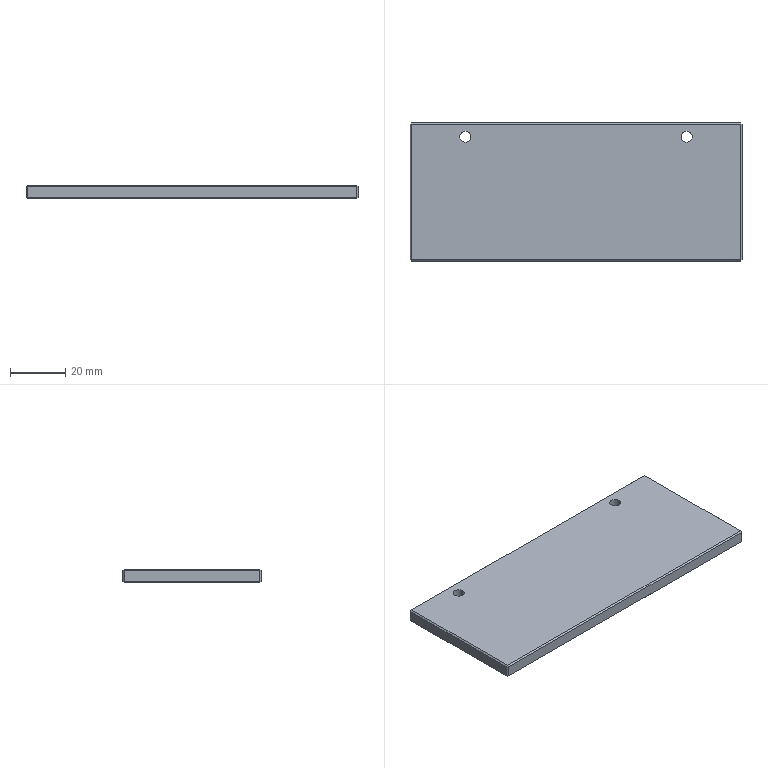Part | SolidWorks | features Chamfer 1, Extrusion 1, HoleWzd 1 | 1 solid | 30 faces | box 120 x 50 x 5 mm | volume 29788 mm3 | plane 26 | cylinder 4 | commonest cylinder face diameters 4 x4
STEP:
#1=CARTESIAN_POINT('',(22.,45.,0.));
#2=VERTEX_POINT('',#1);
#3=CARTESIAN_POINT('',(18.,45.,0.));
#4=VERTEX_POINT('',#3);
#5=CARTESIAN_POINT('',(20.,45.,0.));
#6=DIRECTION('',(0.,0.,-1.));
#7=DIRECTION('',(-1.,0.,0.));
#8=AXIS2_PLACEMENT_3D('',#5,#6,#7);
#9=CIRCLE('',#8,2.);
#10=EDGE_CURVE('',#2,#4,#9,.T.);
#11=ORIENTED_EDGE('',*,*,#10,.T.);
#12=CARTESIAN_POINT('',(18.,45.,5.));
#13=VERTEX_POINT('',#12);
#14=CARTESIAN_POINT('',(18.,45.,5.));
#15=DIRECTION('',(0.,0.,1.));
#16=VECTOR('',#15,1000.);
#17=LINE('',#14,#16);
#18=EDGE_CURVE('',#4,#13,#17,.T.);
#19=ORIENTED_EDGE('',*,*,#18,.T.);
#20=CARTESIAN_POINT('',(22.,45.,5.));
#21=VERTEX_POINT('',#20);
#22=CARTESIAN_POINT('',(20.,45.,5.));
#23=DIRECTION('',(0.,0.,1.));
#24=DIRECTION('',(1.,0.,0.));
#25=AXIS2_PLACEMENT_3D('',#22,#23,#24);
#26=CIRCLE('',#25,2.);
#27=EDGE_CURVE('',#13,#21,#26,.T.);
#28=ORIENTED_EDGE('',*,*,#27,.T.);
#29=CARTESIAN_POINT('',(22.,45.,5.));
#30=DIRECTION('',(0.,0.,1.));
#31=VECTOR('',#30,1000.);
#32=LINE('',#29,#31);
#33=EDGE_CURVE('',#2,#21,#32,.T.);
#34=ORIENTED_EDGE('',*,*,#33,.F.);
#35=EDGE_LOOP('',(#11,#19,#28,#34));
#36=FACE_OUTER_BOUND('',#35,.T.);
#37=CARTESIAN_POINT('',(20.,45.,5.));
#38=DIRECTION('',(0.,0.,1.));
#39=DIRECTION('',(1.,0.,0.));
#40=AXIS2_PLACEMENT_3D('',#37,#38,#39);
#41=CYLINDRICAL_SURFACE('',#40,2.);
#42=ADVANCED_FACE('',(#36),#41,.F.);
#43=CARTESIAN_POINT('',(102.,45.,0.));
#44=VERTEX_POINT('',#43);
#45=CARTESIAN_POINT('',(98.,45.,0.));
#46=VERTEX_POINT('',#45);
#47=CARTESIAN_POINT('',(100.,45.,0.));
#48=DIRECTION('',(0.,0.,-1.));
#49=DIRECTION('',(-1.,0.,0.));
#50=AXIS2_PLACEMENT_3D('',#47,#48,#49);
#51=CIRCLE('',#50,2.);
#52=EDGE_CURVE('',#44,#46,#51,.T.);
#53=ORIENTED_EDGE('',*,*,#52,.T.);
#54=CARTESIAN_POINT('',(98.,45.,5.));
#55=VERTEX_POINT('',#54);
#56=CARTESIAN_POINT('',(98.,45.,5.));
#57=DIRECTION('',(0.,0.,1.));
#58=VECTOR('',#57,1000.);
#59=LINE('',#56,#58);
#60=EDGE_CURVE('',#46,#55,#59,.T.);
#61=ORIENTED_EDGE('',*,*,#60,.T.);
#62=CARTESIAN_POINT('',(102.,45.,5.));
#63=VERTEX_POINT('',#62);
#64=CARTESIAN_POINT('',(100.,45.,5.));
#65=DIRECTION('',(0.,0.,1.));
#66=DIRECTION('',(1.,0.,0.));
#67=AXIS2_PLACEMENT_3D('',#64,#65,#66);
#68=CIRCLE('',#67,2.);
#69=EDGE_CURVE('',#55,#63,#68,.T.);
#70=ORIENTED_EDGE('',*,*,#69,.T.);
#71=CARTESIAN_POINT('',(102.,45.,5.));
#72=DIRECTION('',(0.,0.,1.));
#73=VECTOR('',#72,1000.);
#74=LINE('',#71,#73);
#75=EDGE_CURVE('',#44,#63,#74,.T.);
#76=ORIENTED_EDGE('',*,*,#75,.F.);
#77=EDGE_LOOP('',(#53,#61,#70,#76));
#78=FACE_OUTER_BOUND('',#77,.T.);
#79=CARTESIAN_POINT('',(100.,45.,5.));
#80=DIRECTION('',(0.,0.,1.));
#81=DIRECTION('',(1.,0.,0.));
#82=AXIS2_PLACEMENT_3D('',#79,#80,#81);
#83=CYLINDRICAL_SURFACE('',#82,2.);
#84=ADVANCED_FACE('',(#78),#83,.F.);
#85=CARTESIAN_POINT('',(0.,0.5,4.5));
#86=VERTEX_POINT('',#85);
#87=CARTESIAN_POINT('',(0.,49.5,4.5));
#88=VERTEX_POINT('',#87);
#89=CARTESIAN_POINT('',(0.,0.,4.5));
#90=DIRECTION('',(0.,1.,0.));
#91=VECTOR('',#90,1000.);
#92=LINE('',#89,#91);
#93=EDGE_CURVE('',#86,#88,#92,.T.);
#94=ORIENTED_EDGE('',*,*,#93,.T.);
#95=CARTESIAN_POINT('',(0.,49.5,0.5));
#96=VERTEX_POINT('',#95);
#97=CARTESIAN_POINT('',(0.,49.5,5.));
#98=DIRECTION('',(0.,0.,-1.));
#99=VECTOR('',#98,1000.);
#100=LINE('',#97,#99);
#101=EDGE_CURVE('',#88,#96,#100,.T.);
#102=ORIENTED_EDGE('',*,*,#101,.T.);
#103=CARTESIAN_POINT('',(0.,0.5,0.5));
#104=VERTEX_POINT('',#103);
#105=CARTESIAN_POINT('',(0.,0.,0.5));
#106=DIRECTION('',(0.,-1.,0.));
#107=VECTOR('',#106,1000.);
#108=LINE('',#105,#107);
#109=EDGE_CURVE('',#96,#104,#108,.T.);
#110=ORIENTED_EDGE('',*,*,#109,.T.);
#111=CARTESIAN_POINT('',(0.,0.5,5.));
#112=DIRECTION('',(0.,0.,1.));
#113=VECTOR('',#112,1000.);
#114=LINE('',#111,#113);
#115=EDGE_CURVE('',#104,#86,#114,.T.);
#116=ORIENTED_EDGE('',*,*,#115,.T.);
#117=EDGE_LOOP('',(#94,#102,#110,#116));
#118=FACE_OUTER_BOUND('',#117,.T.);
#119=CARTESIAN_POINT('',(0.,0.,5.));
#120=DIRECTION('',(1.,0.,0.));
#121=DIRECTION('',(0.,0.,-1.));
#122=AXIS2_PLACEMENT_3D('',#119,#120,#121);
#123=PLANE('',#122);
#124=ADVANCED_FACE('',(#118),#123,.F.);
#125=CARTESIAN_POINT('',(119.5,0.,0.5));
#126=VERTEX_POINT('',#125);
#127=CARTESIAN_POINT('',(119.5,0.,4.5));
#128=VERTEX_POINT('',#127);
#129=CARTESIAN_POINT('',(119.5,0.,5.));
#130=DIRECTION('',(0.,0.,1.));
#131=VECTOR('',#130,1000.);
#132=LINE('',#129,#131);
#133=EDGE_CURVE('',#126,#128,#132,.T.);
#134=ORIENTED_EDGE('',*,*,#133,.T.);
#135=CARTESIAN_POINT('',(0.5,0.,4.5));
#136=VERTEX_POINT('',#135);
#137=CARTESIAN_POINT('',(0.,0.,4.5));
#138=DIRECTION('',(-1.,0.,0.));
#139=VECTOR('',#138,1000.);
#140=LINE('',#137,#139);
#141=EDGE_CURVE('',#128,#136,#140,.T.);
#142=ORIENTED_EDGE('',*,*,#141,.T.);
#143=CARTESIAN_POINT('',(0.5,0.,0.5));
#144=VERTEX_POINT('',#143);
#145=CARTESIAN_POINT('',(0.5,0.,5.));
#146=DIRECTION('',(0.,0.,-1.));
#147=VECTOR('',#146,1000.);
#148=LINE('',#145,#147);
#149=EDGE_CURVE('',#136,#144,#148,.T.);
#150=ORIENTED_EDGE('',*,*,#149,.T.);
#151=CARTESIAN_POINT('',(120.,0.,0.5));
#152=DIRECTION('',(1.,0.,0.));
#153=VECTOR('',#152,1000.);
#154=LINE('',#151,#153);
#155=EDGE_CURVE('',#144,#126,#154,.T.);
#156=ORIENTED_EDGE('',*,*,#155,.T.);
#157=EDGE_LOOP('',(#134,#142,#150,#156));
#158=FACE_OUTER_BOUND('',#157,.T.);
#159=CARTESIAN_POINT('',(0.,0.,5.));
#160=DIRECTION('',(0.,1.,0.));
#161=DIRECTION('',(0.,0.,1.));
#162=AXIS2_PLACEMENT_3D('',#159,#160,#161);
#163=PLANE('',#162);
#164=ADVANCED_FACE('',(#158),#163,.F.);
#165=CARTESIAN_POINT('',(120.,49.5,4.5));
#166=VERTEX_POINT('',#165);
#167=CARTESIAN_POINT('',(120.,0.5,4.5));
#168=VERTEX_POINT('',#167);
#169=CARTESIAN_POINT('',(120.,0.,4.5));
#170=DIRECTION('',(0.,-1.,0.));
#171=VECTOR('',#170,1000.);
#172=LINE('',#169,#171);
#173=EDGE_CURVE('',#166,#168,#172,.T.);
#174=ORIENTED_EDGE('',*,*,#173,.T.);
#175=CARTESIAN_POINT('',(120.,0.5,0.5));
#176=VERTEX_POINT('',#175);
#177=CARTESIAN_POINT('',(120.,0.5,5.));
#178=DIRECTION('',(0.,0.,-1.));
#179=VECTOR('',#178,1000.);
#180=LINE('',#177,#179);
#181=EDGE_CURVE('',#168,#176,#180,.T.);
#182=ORIENTED_EDGE('',*,*,#181,.T.);
#183=CARTESIAN_POINT('',(120.,49.5,0.5));
#184=VERTEX_POINT('',#183);
#185=CARTESIAN_POINT('',(120.,50.,0.5));
#186=DIRECTION('',(0.,1.,0.));
#187=VECTOR('',#186,1000.);
#188=LINE('',#185,#187);
#189=EDGE_CURVE('',#176,#184,#188,.T.);
#190=ORIENTED_EDGE('',*,*,#189,.T.);
#191=CARTESIAN_POINT('',(120.,49.5,5.));
#192=DIRECTION('',(0.,0.,1.));
#193=VECTOR('',#192,1000.);
#194=LINE('',#191,#193);
#195=EDGE_CURVE('',#184,#166,#194,.T.);
#196=ORIENTED_EDGE('',*,*,#195,.T.);
#197=EDGE_LOOP('',(#174,#182,#190,#196));
#198=FACE_OUTER_BOUND('',#197,.T.);
#199=CARTESIAN_POINT('',(120.,0.,5.));
#200=DIRECTION('',(-1.,0.,0.));
#201=DIRECTION('',(0.,0.,1.));
#202=AXIS2_PLACEMENT_3D('',#199,#200,#201);
#203=PLANE('',#202);
#204=ADVANCED_FACE('',(#198),#203,.F.);
#205=CARTESIAN_POINT('',(0.5,50.,4.5));
#206=VERTEX_POINT('',#205);
#207=CARTESIAN_POINT('',(119.5,50.,4.5));
#208=VERTEX_POINT('',#207);
#209=CARTESIAN_POINT('',(0.,50.,4.5));
#210=DIRECTION('',(1.,0.,0.));
#211=VECTOR('',#210,1000.);
#212=LINE('',#209,#211);
#213=EDGE_CURVE('',#206,#208,#212,.T.);
#214=ORIENTED_EDGE('',*,*,#213,.T.);
#215=CARTESIAN_POINT('',(119.5,50.,0.5));
#216=VERTEX_POINT('',#215);
#217=CARTESIAN_POINT('',(119.5,50.,5.));
#218=DIRECTION('',(0.,0.,-1.));
#219=VECTOR('',#218,1000.);
#220=LINE('',#217,#219);
#221=EDGE_CURVE('',#208,#216,#220,.T.);
#222=ORIENTED_EDGE('',*,*,#221,.T.);
#223=CARTESIAN_POINT('',(0.5,50.,0.5));
#224=VERTEX_POINT('',#223);
#225=CARTESIAN_POINT('',(0.,50.,0.5));
#226=DIRECTION('',(-1.,0.,0.));
#227=VECTOR('',#226,1000.);
#228=LINE('',#225,#227);
#229=EDGE_CURVE('',#216,#224,#228,.T.);
#230=ORIENTED_EDGE('',*,*,#229,.T.);
#231=CARTESIAN_POINT('',(0.5,50.,5.));
#232=DIRECTION('',(0.,0.,1.));
#233=VECTOR('',#232,1000.);
#234=LINE('',#231,#233);
#235=EDGE_CURVE('',#224,#206,#234,.T.);
#236=ORIENTED_EDGE('',*,*,#235,.T.);
#237=EDGE_LOOP('',(#214,#222,#230,#236));
#238=FACE_OUTER_BOUND('',#237,.T.);
#239=CARTESIAN_POINT('',(0.,50.,5.));
#240=DIRECTION('',(0.,-1.,0.));
#241=DIRECTION('',(0.,0.,-1.));
#242=AXIS2_PLACEMENT_3D('',#239,#240,#241);
#243=PLANE('',#242);
#244=ADVANCED_FACE('',(#238),#243,.F.);
#245=CARTESIAN_POINT('',(0.5,0.5,5.));
#246=VERTEX_POINT('',#245);
#247=CARTESIAN_POINT('',(119.5,0.5,5.));
#248=VERTEX_POINT('',#247);
#249=CARTESIAN_POINT('',(0.,0.5,5.));
#250=DIRECTION('',(1.,0.,0.));
#251=VECTOR('',#250,1000.);
#252=LINE('',#249,#251);
#253=EDGE_CURVE('',#246,#248,#252,.T.);
#254=ORIENTED_EDGE('',*,*,#253,.T.);
#255=CARTESIAN_POINT('',(119.5,49.5,5.));
#256=VERTEX_POINT('',#255);
#257=CARTESIAN_POINT('',(119.5,0.,5.));
#258=DIRECTION('',(0.,1.,0.));
#259=VECTOR('',#258,1000.);
#260=LINE('',#257,#259);
#261=EDGE_CURVE('',#248,#256,#260,.T.);
#262=ORIENTED_EDGE('',*,*,#261,.T.);
#263=CARTESIAN_POINT('',(0.5,49.5,5.));
#264=VERTEX_POINT('',#263);
#265=CARTESIAN_POINT('',(0.,49.5,5.));
#266=DIRECTION('',(-1.,0.,0.));
#267=VECTOR('',#266,1000.);
#268=LINE('',#265,#267);
#269=EDGE_CURVE('',#256,#264,#268,.T.);
#270=ORIENTED_EDGE('',*,*,#269,.T.);
#271=CARTESIAN_POINT('',(0.5,0.,5.));
#272=DIRECTION('',(0.,-1.,0.));
#273=VECTOR('',#272,1000.);
#274=LINE('',#271,#273);
#275=EDGE_CURVE('',#264,#246,#274,.T.);
#276=ORIENTED_EDGE('',*,*,#275,.T.);
#277=EDGE_LOOP('',(#254,#262,#270,#276));
#278=FACE_OUTER_BOUND('',#277,.T.);
#279=CARTESIAN_POINT('',(20.,45.,5.));
#280=DIRECTION('',(0.,0.,1.));
#281=DIRECTION('',(1.,0.,0.));
#282=AXIS2_PLACEMENT_3D('',#279,#280,#281);
#283=CIRCLE('',#282,2.);
#284=EDGE_CURVE('',#21,#13,#283,.T.);
#285=ORIENTED_EDGE('',*,*,#284,.F.);
#286=ORIENTED_EDGE('',*,*,#27,.F.);
#287=EDGE_LOOP('',(#285,#286));
#288=FACE_BOUND('',#287,.T.);
#289=CARTESIAN_POINT('',(100.,45.,5.));
#290=DIRECTION('',(0.,0.,1.));
#291=DIRECTION('',(1.,0.,0.));
#292=AXIS2_PLACEMENT_3D('',#289,#290,#291);
#293=CIRCLE('',#292,2.);
#294=EDGE_CURVE('',#63,#55,#293,.T.);
#295=ORIENTED_EDGE('',*,*,#294,.F.);
#296=ORIENTED_EDGE('',*,*,#69,.F.);
#297=EDGE_LOOP('',(#295,#296));
#298=FACE_BOUND('',#297,.T.);
#299=CARTESIAN_POINT('',(0.,0.,5.));
#300=DIRECTION('',(0.,0.,-1.));
#301=DIRECTION('',(-1.,0.,0.));
#302=AXIS2_PLACEMENT_3D('',#299,#300,#301);
#303=PLANE('',#302);
#304=ADVANCED_FACE('',(#278,#288,#298),#303,.F.);
#305=CARTESIAN_POINT('',(0.5,49.5,0.));
#306=VERTEX_POINT('',#305);
#307=CARTESIAN_POINT('',(119.5,49.5,0.));
#308=VERTEX_POINT('',#307);
#309=CARTESIAN_POINT('',(120.,49.5,0.));
#310=DIRECTION('',(1.,0.,0.));
#311=VECTOR('',#310,1000.);
#312=LINE('',#309,#311);
#313=EDGE_CURVE('',#306,#308,#312,.T.);
#314=ORIENTED_EDGE('',*,*,#313,.T.);
#315=CARTESIAN_POINT('',(119.5,0.5,0.));
#316=VERTEX_POINT('',#315);
#317=CARTESIAN_POINT('',(119.5,0.,0.));
#318=DIRECTION('',(0.,-1.,0.));
#319=VECTOR('',#318,1000.);
#320=LINE('',#317,#319);
#321=EDGE_CURVE('',#308,#316,#320,.T.);
#322=ORIENTED_EDGE('',*,*,#321,.T.);
#323=CARTESIAN_POINT('',(0.5,0.5,0.));
#324=VERTEX_POINT('',#323);
#325=CARTESIAN_POINT('',(0.,0.5,0.));
#326=DIRECTION('',(-1.,0.,0.));
#327=VECTOR('',#326,1000.);
#328=LINE('',#325,#327);
#329=EDGE_CURVE('',#316,#324,#328,.T.);
#330=ORIENTED_EDGE('',*,*,#329,.T.);
#331=CARTESIAN_POINT('',(0.5,50.,0.));
#332=DIRECTION('',(0.,1.,0.));
#333=VECTOR('',#332,1000.);
#334=LINE('',#331,#333);
#335=EDGE_CURVE('',#324,#306,#334,.T.);
#336=ORIENTED_EDGE('',*,*,#335,.T.);
#337=EDGE_LOOP('',(#314,#322,#330,#336));
#338=FACE_OUTER_BOUND('',#337,.T.);
#339=ORIENTED_EDGE('',*,*,#10,.F.);
#340=CARTESIAN_POINT('',(20.,45.,0.));
#341=DIRECTION('',(0.,0.,-1.));
#342=DIRECTION('',(-1.,0.,0.));
#343=AXIS2_PLACEMENT_3D('',#340,#341,#342);
#344=CIRCLE('',#343,2.);
#345=EDGE_CURVE('',#4,#2,#344,.T.);
#346=ORIENTED_EDGE('',*,*,#345,.F.);
#347=EDGE_LOOP('',(#339,#346));
#348=FACE_BOUND('',#347,.T.);
#349=ORIENTED_EDGE('',*,*,#52,.F.);
#350=CARTESIAN_POINT('',(100.,45.,0.));
#351=DIRECTION('',(0.,0.,-1.));
#352=DIRECTION('',(-1.,0.,0.));
#353=AXIS2_PLACEMENT_3D('',#350,#351,#352);
#354=CIRCLE('',#353,2.);
#355=EDGE_CURVE('',#46,#44,#354,.T.);
#356=ORIENTED_EDGE('',*,*,#355,.F.);
#357=EDGE_LOOP('',(#349,#356));
#358=FACE_BOUND('',#357,.T.);
#359=CARTESIAN_POINT('',(0.,0.,0.));
#360=DIRECTION('',(0.,0.,-1.));
#361=DIRECTION('',(-1.,0.,0.));
#362=AXIS2_PLACEMENT_3D('',#359,#360,#361);
#363=PLANE('',#362);
#364=ADVANCED_FACE('',(#338,#348,#358),#363,.T.);
#365=ORIENTED_EDGE('',*,*,#60,.F.);
#366=ORIENTED_EDGE('',*,*,#355,.T.);
#367=ORIENTED_EDGE('',*,*,#75,.T.);
#368=ORIENTED_EDGE('',*,*,#294,.T.);
#369=EDGE_LOOP('',(#365,#366,#367,#368));
#370=FACE_OUTER_BOUND('',#369,.T.);
#371=CARTESIAN_POINT('',(100.,45.,5.));
#372=DIRECTION('',(0.,0.,1.));
#373=DIRECTION('',(1.,0.,0.));
#374=AXIS2_PLACEMENT_3D('',#371,#372,#373);
#375=CYLINDRICAL_SURFACE('',#374,2.);
#376=ADVANCED_FACE('',(#370),#375,.F.);
#377=ORIENTED_EDGE('',*,*,#18,.F.);
#378=ORIENTED_EDGE('',*,*,#345,.T.);
#379=ORIENTED_EDGE('',*,*,#33,.T.);
#380=ORIENTED_EDGE('',*,*,#284,.T.);
#381=EDGE_LOOP('',(#377,#378,#379,#380));
#382=FACE_OUTER_BOUND('',#381,.T.);
#383=CARTESIAN_POINT('',(20.,45.,5.));
#384=DIRECTION('',(0.,0.,1.));
#385=DIRECTION('',(1.,0.,0.));
#386=AXIS2_PLACEMENT_3D('',#383,#384,#385);
#387=CYLINDRICAL_SURFACE('',#386,2.);
#388=ADVANCED_FACE('',(#382),#387,.F.);
#389=CARTESIAN_POINT('',(0.5,0.5,0.));
#390=DIRECTION('',(0.7071,0.,-0.7071));
#391=VECTOR('',#390,1000.);
#392=LINE('',#389,#391);
#393=EDGE_CURVE('',#104,#324,#392,.T.);
#394=ORIENTED_EDGE('',*,*,#393,.F.);
#395=ORIENTED_EDGE('',*,*,#109,.F.);
#396=CARTESIAN_POINT('',(0.25,49.5,0.25));
#397=DIRECTION('',(-0.7071,0.,0.7071));
#398=VECTOR('',#397,1000.);
#399=LINE('',#396,#398);
#400=EDGE_CURVE('',#306,#96,#399,.T.);
#401=ORIENTED_EDGE('',*,*,#400,.F.);
#402=ORIENTED_EDGE('',*,*,#335,.F.);
#403=EDGE_LOOP('',(#394,#395,#401,#402));
#404=FACE_OUTER_BOUND('',#403,.T.);
#405=CARTESIAN_POINT('',(0.,0.,0.5));
#406=DIRECTION('',(-0.7071,0.,-0.7071));
#407=DIRECTION('',(0.,1.,0.));
#408=AXIS2_PLACEMENT_3D('',#405,#406,#407);
#409=PLANE('',#408);
#410=ADVANCED_FACE('',(#404),#409,.T.);
#411=CARTESIAN_POINT('',(0.25,0.25,0.5));
#412=DIRECTION('',(0.7071,-0.7071,0.));
#413=VECTOR('',#412,1000.);
#414=LINE('',#411,#413);
#415=EDGE_CURVE('',#104,#144,#414,.T.);
#416=ORIENTED_EDGE('',*,*,#415,.F.);
#417=ORIENTED_EDGE('',*,*,#393,.T.);
#418=CARTESIAN_POINT('',(0.5,0.5,0.));
#419=DIRECTION('',(0.,0.7071,-0.7071));
#420=VECTOR('',#419,1000.);
#421=LINE('',#418,#420);
#422=EDGE_CURVE('',#144,#324,#421,.T.);
#423=ORIENTED_EDGE('',*,*,#422,.F.);
#424=EDGE_LOOP('',(#416,#417,#423));
#425=FACE_OUTER_BOUND('',#424,.T.);
#426=CARTESIAN_POINT('',(0.5,0.5,0.));
#427=DIRECTION('',(-0.5774,-0.5774,-0.5774));
#428=DIRECTION('',(-0.7071,0.,0.7071));
#429=AXIS2_PLACEMENT_3D('',#426,#427,#428);
#430=PLANE('',#429);
#431=ADVANCED_FACE('',(#425),#430,.T.);
#432=CARTESIAN_POINT('',(0.5,50.,0.5));
#433=DIRECTION('',(0.,0.7071,0.7071));
#434=VECTOR('',#433,1000.);
#435=LINE('',#432,#434);
#436=EDGE_CURVE('',#306,#224,#435,.T.);
#437=ORIENTED_EDGE('',*,*,#436,.F.);
#438=ORIENTED_EDGE('',*,*,#400,.T.);
#439=CARTESIAN_POINT('',(0.5,50.,0.5));
#440=DIRECTION('',(-0.7071,-0.7071,0.));
#441=VECTOR('',#440,1000.);
#442=LINE('',#439,#441);
#443=EDGE_CURVE('',#224,#96,#442,.T.);
#444=ORIENTED_EDGE('',*,*,#443,.F.);
#445=EDGE_LOOP('',(#437,#438,#444));
#446=FACE_OUTER_BOUND('',#445,.T.);
#447=CARTESIAN_POINT('',(0.5,50.,0.5));
#448=DIRECTION('',(-0.5774,0.5774,-0.5774));
#449=DIRECTION('',(-0.7071,0.,0.7071));
#450=AXIS2_PLACEMENT_3D('',#447,#448,#449);
#451=PLANE('',#450);
#452=ADVANCED_FACE('',(#446),#451,.T.);
#453=ORIENTED_EDGE('',*,*,#422,.T.);
#454=ORIENTED_EDGE('',*,*,#329,.F.);
#455=CARTESIAN_POINT('',(119.5,0.5,0.));
#456=DIRECTION('',(0.,0.7071,-0.7071));
#457=VECTOR('',#456,1000.);
#458=LINE('',#455,#457);
#459=EDGE_CURVE('',#126,#316,#458,.T.);
#460=ORIENTED_EDGE('',*,*,#459,.F.);
#461=ORIENTED_EDGE('',*,*,#155,.F.);
#462=EDGE_LOOP('',(#453,#454,#460,#461));
#463=FACE_OUTER_BOUND('',#462,.T.);
#464=CARTESIAN_POINT('',(0.,0.,0.5));
#465=DIRECTION('',(0.,-0.7071,-0.7071));
#466=DIRECTION('',(-1.,0.,0.));
#467=AXIS2_PLACEMENT_3D('',#464,#465,#466);
#468=PLANE('',#467);
#469=ADVANCED_FACE('',(#463),#468,.T.);
#470=ORIENTED_EDGE('',*,*,#415,.T.);
#471=ORIENTED_EDGE('',*,*,#149,.F.);
#472=CARTESIAN_POINT('',(0.5,0.,4.5));
#473=DIRECTION('',(0.7071,-0.7071,0.));
#474=VECTOR('',#473,1000.);
#475=LINE('',#472,#474);
#476=EDGE_CURVE('',#86,#136,#475,.T.);
#477=ORIENTED_EDGE('',*,*,#476,.F.);
#478=ORIENTED_EDGE('',*,*,#115,.F.);
#479=EDGE_LOOP('',(#470,#471,#477,#478));
#480=FACE_OUTER_BOUND('',#479,.T.);
#481=CARTESIAN_POINT('',(0.5,0.,5.));
#482=DIRECTION('',(0.7071,0.7071,0.));
#483=DIRECTION('',(0.,0.,-1.));
#484=AXIS2_PLACEMENT_3D('',#481,#482,#483);
#485=PLANE('',#484);
#486=ADVANCED_FACE('',(#480),#485,.F.);
#487=CARTESIAN_POINT('',(0.5,49.5,5.));
#488=DIRECTION('',(0.7071,0.,0.7071));
#489=VECTOR('',#488,1000.);
#490=LINE('',#487,#489);
#491=EDGE_CURVE('',#88,#264,#490,.T.);
#492=ORIENTED_EDGE('',*,*,#491,.F.);
#493=ORIENTED_EDGE('',*,*,#93,.F.);
#494=CARTESIAN_POINT('',(0.25,0.5,4.75));
#495=DIRECTION('',(-0.7071,0.,-0.7071));
#496=VECTOR('',#495,1000.);
#497=LINE('',#494,#496);
#498=EDGE_CURVE('',#246,#86,#497,.T.);
#499=ORIENTED_EDGE('',*,*,#498,.F.);
#500=ORIENTED_EDGE('',*,*,#275,.F.);
#501=EDGE_LOOP('',(#492,#493,#499,#500));
#502=FACE_OUTER_BOUND('',#501,.T.);
#503=CARTESIAN_POINT('',(0.5,0.,5.));
#504=DIRECTION('',(0.7071,0.,-0.7071));
#505=DIRECTION('',(0.,-1.,0.));
#506=AXIS2_PLACEMENT_3D('',#503,#504,#505);
#507=PLANE('',#506);
#508=ADVANCED_FACE('',(#502),#507,.F.);
#509=ORIENTED_EDGE('',*,*,#443,.T.);
#510=ORIENTED_EDGE('',*,*,#101,.F.);
#511=CARTESIAN_POINT('',(0.25,49.75,4.5));
#512=DIRECTION('',(-0.7071,-0.7071,0.));
#513=VECTOR('',#512,1000.);
#514=LINE('',#511,#513);
#515=EDGE_CURVE('',#206,#88,#514,.T.);
#516=ORIENTED_EDGE('',*,*,#515,.F.);
#517=ORIENTED_EDGE('',*,*,#235,.F.);
#518=EDGE_LOOP('',(#509,#510,#516,#517));
#519=FACE_OUTER_BOUND('',#518,.T.);
#520=CARTESIAN_POINT('',(0.,49.5,5.));
#521=DIRECTION('',(0.7071,-0.7071,0.));
#522=DIRECTION('',(0.,0.,-1.));
#523=AXIS2_PLACEMENT_3D('',#520,#521,#522);
#524=PLANE('',#523);
#525=ADVANCED_FACE('',(#519),#524,.F.);
#526=ORIENTED_EDGE('',*,*,#436,.T.);
#527=ORIENTED_EDGE('',*,*,#229,.F.);
#528=CARTESIAN_POINT('',(119.5,49.75,0.25));
#529=DIRECTION('',(0.,0.7071,0.7071));
#530=VECTOR('',#529,1000.);
#531=LINE('',#528,#530);
#532=EDGE_CURVE('',#308,#216,#531,.T.);
#533=ORIENTED_EDGE('',*,*,#532,.F.);
#534=ORIENTED_EDGE('',*,*,#313,.F.);
#535=EDGE_LOOP('',(#526,#527,#533,#534));
#536=FACE_OUTER_BOUND('',#535,.T.);
#537=CARTESIAN_POINT('',(0.,50.,0.5));
#538=DIRECTION('',(0.,0.7071,-0.7071));
#539=DIRECTION('',(1.,0.,0.));
#540=AXIS2_PLACEMENT_3D('',#537,#538,#539);
#541=PLANE('',#540);
#542=ADVANCED_FACE('',(#536),#541,.T.);
#543=CARTESIAN_POINT('',(119.5,0.5,0.));
#544=DIRECTION('',(0.7071,0.,0.7071));
#545=VECTOR('',#544,1000.);
#546=LINE('',#543,#545);
#547=EDGE_CURVE('',#316,#176,#546,.T.);
#548=ORIENTED_EDGE('',*,*,#547,.F.);
#549=ORIENTED_EDGE('',*,*,#321,.F.);
#550=CARTESIAN_POINT('',(120.,49.5,0.5));
#551=DIRECTION('',(-0.7071,0.,-0.7071));
#552=VECTOR('',#551,1000.);
#553=LINE('',#550,#552);
#554=EDGE_CURVE('',#184,#308,#553,.T.);
#555=ORIENTED_EDGE('',*,*,#554,.F.);
#556=ORIENTED_EDGE('',*,*,#189,.F.);
#557=EDGE_LOOP('',(#548,#549,#555,#556));
#558=FACE_OUTER_BOUND('',#557,.T.);
#559=CARTESIAN_POINT('',(120.,0.,0.5));
#560=DIRECTION('',(0.7071,0.,-0.7071));
#561=DIRECTION('',(0.,-1.,0.));
#562=AXIS2_PLACEMENT_3D('',#559,#560,#561);
#563=PLANE('',#562);
#564=ADVANCED_FACE('',(#558),#563,.T.);
#565=ORIENTED_EDGE('',*,*,#459,.T.);
#566=ORIENTED_EDGE('',*,*,#547,.T.);
#567=CARTESIAN_POINT('',(119.75,0.25,0.5));
#568=DIRECTION('',(0.7071,0.7071,0.));
#569=VECTOR('',#568,1000.);
#570=LINE('',#567,#569);
#571=EDGE_CURVE('',#126,#176,#570,.T.);
#572=ORIENTED_EDGE('',*,*,#571,.F.);
#573=EDGE_LOOP('',(#565,#566,#572));
#574=FACE_OUTER_BOUND('',#573,.T.);
#575=CARTESIAN_POINT('',(119.5,0.5,0.));
#576=DIRECTION('',(0.5774,-0.5774,-0.5774));
#577=DIRECTION('',(-0.7071,0.,-0.7071));
#578=AXIS2_PLACEMENT_3D('',#575,#576,#577);
#579=PLANE('',#578);
#580=ADVANCED_FACE('',(#574),#579,.T.);
#581=ORIENTED_EDGE('',*,*,#498,.T.);
#582=ORIENTED_EDGE('',*,*,#476,.T.);
#583=CARTESIAN_POINT('',(0.5,0.,4.5));
#584=DIRECTION('',(0.,-0.7071,-0.7071));
#585=VECTOR('',#584,1000.);
#586=LINE('',#583,#585);
#587=EDGE_CURVE('',#246,#136,#586,.T.);
#588=ORIENTED_EDGE('',*,*,#587,.F.);
#589=EDGE_LOOP('',(#581,#582,#588));
#590=FACE_OUTER_BOUND('',#589,.T.);
#591=CARTESIAN_POINT('',(0.5,0.,4.5));
#592=DIRECTION('',(-0.5774,-0.5774,0.5774));
#593=DIRECTION('',(0.7071,0.,0.7071));
#594=AXIS2_PLACEMENT_3D('',#591,#592,#593);
#595=PLANE('',#594);
#596=ADVANCED_FACE('',(#590),#595,.T.);
#597=ORIENTED_EDGE('',*,*,#515,.T.);
#598=ORIENTED_EDGE('',*,*,#491,.T.);
#599=CARTESIAN_POINT('',(0.5,49.5,5.));
#600=DIRECTION('',(0.,-0.7071,0.7071));
#601=VECTOR('',#600,1000.);
#602=LINE('',#599,#601);
#603=EDGE_CURVE('',#206,#264,#602,.T.);
#604=ORIENTED_EDGE('',*,*,#603,.F.);
#605=EDGE_LOOP('',(#597,#598,#604));
#606=FACE_OUTER_BOUND('',#605,.T.);
#607=CARTESIAN_POINT('',(0.5,49.5,5.));
#608=DIRECTION('',(-0.5774,0.5774,0.5774));
#609=DIRECTION('',(0.7071,0.,0.7071));
#610=AXIS2_PLACEMENT_3D('',#607,#608,#609);
#611=PLANE('',#610);
#612=ADVANCED_FACE('',(#606),#611,.T.);
#613=ORIENTED_EDGE('',*,*,#554,.T.);
#614=ORIENTED_EDGE('',*,*,#532,.T.);
#615=CARTESIAN_POINT('',(120.,49.5,0.5));
#616=DIRECTION('',(-0.7071,0.7071,0.));
#617=VECTOR('',#616,1000.);
#618=LINE('',#615,#617);
#619=EDGE_CURVE('',#184,#216,#618,.T.);
#620=ORIENTED_EDGE('',*,*,#619,.F.);
#621=EDGE_LOOP('',(#613,#614,#620));
#622=FACE_OUTER_BOUND('',#621,.T.);
#623=CARTESIAN_POINT('',(120.,49.5,0.5));
#624=DIRECTION('',(0.5774,0.5774,-0.5774));
#625=DIRECTION('',(-0.7071,0.,-0.7071));
#626=AXIS2_PLACEMENT_3D('',#623,#624,#625);
#627=PLANE('',#626);
#628=ADVANCED_FACE('',(#622),#627,.T.);
#629=ORIENTED_EDGE('',*,*,#571,.T.);
#630=ORIENTED_EDGE('',*,*,#181,.F.);
#631=CARTESIAN_POINT('',(120.,0.5,4.5));
#632=DIRECTION('',(0.7071,0.7071,0.));
#633=VECTOR('',#632,1000.);
#634=LINE('',#631,#633);
#635=EDGE_CURVE('',#128,#168,#634,.T.);
#636=ORIENTED_EDGE('',*,*,#635,.F.);
#637=ORIENTED_EDGE('',*,*,#133,.F.);
#638=EDGE_LOOP('',(#629,#630,#636,#637));
#639=FACE_OUTER_BOUND('',#638,.T.);
#640=CARTESIAN_POINT('',(120.,0.5,5.));
#641=DIRECTION('',(-0.7071,0.7071,0.));
#642=DIRECTION('',(0.,0.,-1.));
#643=AXIS2_PLACEMENT_3D('',#640,#641,#642);
#644=PLANE('',#643);
#645=ADVANCED_FACE('',(#639),#644,.F.);
#646=ORIENTED_EDGE('',*,*,#587,.T.);
#647=ORIENTED_EDGE('',*,*,#141,.F.);
#648=CARTESIAN_POINT('',(119.5,0.25,4.75));
#649=DIRECTION('',(0.,-0.7071,-0.7071));
#650=VECTOR('',#649,1000.);
#651=LINE('',#648,#650);
#652=EDGE_CURVE('',#248,#128,#651,.T.);
#653=ORIENTED_EDGE('',*,*,#652,.F.);
#654=ORIENTED_EDGE('',*,*,#253,.F.);
#655=EDGE_LOOP('',(#646,#647,#653,#654));
#656=FACE_OUTER_BOUND('',#655,.T.);
#657=CARTESIAN_POINT('',(0.,0.5,5.));
#658=DIRECTION('',(0.,0.7071,-0.7071));
#659=DIRECTION('',(1.,0.,0.));
#660=AXIS2_PLACEMENT_3D('',#657,#658,#659);
#661=PLANE('',#660);
#662=ADVANCED_FACE('',(#656),#661,.F.);
#663=ORIENTED_EDGE('',*,*,#603,.T.);
#664=ORIENTED_EDGE('',*,*,#269,.F.);
#665=CARTESIAN_POINT('',(119.5,49.5,5.));
#666=DIRECTION('',(0.,-0.7071,0.7071));
#667=VECTOR('',#666,1000.);
#668=LINE('',#665,#667);
#669=EDGE_CURVE('',#208,#256,#668,.T.);
#670=ORIENTED_EDGE('',*,*,#669,.F.);
#671=ORIENTED_EDGE('',*,*,#213,.F.);
#672=EDGE_LOOP('',(#663,#664,#670,#671));
#673=FACE_OUTER_BOUND('',#672,.T.);
#674=CARTESIAN_POINT('',(0.,49.5,5.));
#675=DIRECTION('',(0.,-0.7071,-0.7071));
#676=DIRECTION('',(-1.,0.,0.));
#677=AXIS2_PLACEMENT_3D('',#674,#675,#676);
#678=PLANE('',#677);
#679=ADVANCED_FACE('',(#673),#678,.F.);
#680=ORIENTED_EDGE('',*,*,#619,.T.);
#681=ORIENTED_EDGE('',*,*,#221,.F.);
#682=CARTESIAN_POINT('',(119.75,49.75,4.5));
#683=DIRECTION('',(-0.7071,0.7071,0.));
#684=VECTOR('',#683,1000.);
#685=LINE('',#682,#684);
#686=EDGE_CURVE('',#166,#208,#685,.T.);
#687=ORIENTED_EDGE('',*,*,#686,.F.);
#688=ORIENTED_EDGE('',*,*,#195,.F.);
#689=EDGE_LOOP('',(#680,#681,#687,#688));
#690=FACE_OUTER_BOUND('',#689,.T.);
#691=CARTESIAN_POINT('',(119.5,50.,5.));
#692=DIRECTION('',(-0.7071,-0.7071,0.));
#693=DIRECTION('',(0.,0.,-1.));
#694=AXIS2_PLACEMENT_3D('',#691,#692,#693);
#695=PLANE('',#694);
#696=ADVANCED_FACE('',(#690),#695,.F.);
#697=ORIENTED_EDGE('',*,*,#652,.T.);
#698=ORIENTED_EDGE('',*,*,#635,.T.);
#699=CARTESIAN_POINT('',(120.,0.5,4.5));
#700=DIRECTION('',(0.7071,0.,-0.7071));
#701=VECTOR('',#700,1000.);
#702=LINE('',#699,#701);
#703=EDGE_CURVE('',#248,#168,#702,.T.);
#704=ORIENTED_EDGE('',*,*,#703,.F.);
#705=EDGE_LOOP('',(#697,#698,#704));
#706=FACE_OUTER_BOUND('',#705,.T.);
#707=CARTESIAN_POINT('',(120.,0.5,4.5));
#708=DIRECTION('',(0.5774,-0.5774,0.5774));
#709=DIRECTION('',(0.7071,0.,-0.7071));
#710=AXIS2_PLACEMENT_3D('',#707,#708,#709);
#711=PLANE('',#710);
#712=ADVANCED_FACE('',(#706),#711,.T.);
#713=ORIENTED_EDGE('',*,*,#686,.T.);
#714=ORIENTED_EDGE('',*,*,#669,.T.);
#715=CARTESIAN_POINT('',(119.5,49.5,5.));
#716=DIRECTION('',(-0.7071,0.,0.7071));
#717=VECTOR('',#716,1000.);
#718=LINE('',#715,#717);
#719=EDGE_CURVE('',#166,#256,#718,.T.);
#720=ORIENTED_EDGE('',*,*,#719,.F.);
#721=EDGE_LOOP('',(#713,#714,#720));
#722=FACE_OUTER_BOUND('',#721,.T.);
#723=CARTESIAN_POINT('',(119.5,49.5,5.));
#724=DIRECTION('',(0.5774,0.5774,0.5774));
#725=DIRECTION('',(0.7071,0.,-0.7071));
#726=AXIS2_PLACEMENT_3D('',#723,#724,#725);
#727=PLANE('',#726);
#728=ADVANCED_FACE('',(#722),#727,.T.);
#729=ORIENTED_EDGE('',*,*,#703,.T.);
#730=ORIENTED_EDGE('',*,*,#173,.F.);
#731=ORIENTED_EDGE('',*,*,#719,.T.);
#732=ORIENTED_EDGE('',*,*,#261,.F.);
#733=EDGE_LOOP('',(#729,#730,#731,#732));
#734=FACE_OUTER_BOUND('',#733,.T.);
#735=CARTESIAN_POINT('',(119.5,0.,5.));
#736=DIRECTION('',(-0.7071,0.,-0.7071));
#737=DIRECTION('',(0.,1.,0.));
#738=AXIS2_PLACEMENT_3D('',#735,#736,#737);
#739=PLANE('',#738);
#740=ADVANCED_FACE('',(#734),#739,.F.);
#741=CLOSED_SHELL('',(#42,#84,#124,#164,#204,#244,#304,#364,#376,#388,#410,#431,#452,#469,#486,#508,#525,#542,#564,#580,#596,#612,#628,#645,#662,#679,#696,#712,#728,#740));
#742=MANIFOLD_SOLID_BREP('',#741);
#743=CARTESIAN_POINT('',(0.,0.,0.));
#744=DIRECTION('',(0.,0.,1.));
#745=DIRECTION('',(1.,0.,0.));
#746=AXIS2_PLACEMENT_3D('',#743,#744,#745);
#747=(LENGTH_UNIT()NAMED_UNIT(*)SI_UNIT(.MILLI.,.METRE.));
#748=UNCERTAINTY_MEASURE_WITH_UNIT(LENGTH_MEASURE(0.00001),#747,'','');
#749=(NAMED_UNIT(*)PLANE_ANGLE_UNIT()SI_UNIT($,.RADIAN.));
#750=(NAMED_UNIT(*)SI_UNIT($,.STERADIAN.)SOLID_ANGLE_UNIT());
#751=(GEOMETRIC_REPRESENTATION_CONTEXT(3)GLOBAL_UNCERTAINTY_ASSIGNED_CONTEXT((#748))GLOBAL_UNIT_ASSIGNED_CONTEXT((#747,#749,#750))REPRESENTATION_CONTEXT('',''));
#752=ADVANCED_BREP_SHAPE_REPRESENTATION('',(#742,#746),#751);